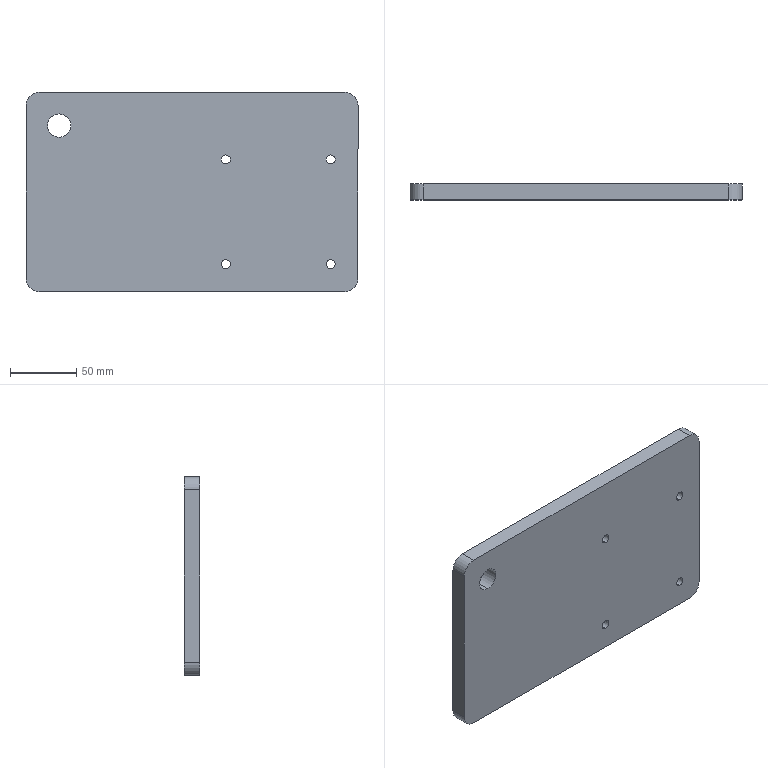Part | SolidWorks | features HoleWzd 4, ICE 2, Extrusion 1, Fillet 1 | 1 solid | 20 faces | box 250 x 12 x 150 mm | volume 444340 mm3 | cylinder 14 | plane 6 | commonest cylinder face diameters 6.8 x8 20 x4 17.5 x2
STEP:
#1=CARTESIAN_POINT('',(25.5,0.,-57.9));
#2=VERTEX_POINT('',#1);
#3=CARTESIAN_POINT('',(25.5,0.,-51.1));
#4=VERTEX_POINT('',#3);
#5=CARTESIAN_POINT('',(25.5,0.,-54.5));
#6=DIRECTION('',(0.,1.,0.));
#7=DIRECTION('',(0.,0.,1.));
#8=AXIS2_PLACEMENT_3D('',#5,#6,#7);
#9=CIRCLE('',#8,3.4);
#10=EDGE_CURVE('',#2,#4,#9,.T.);
#11=ORIENTED_EDGE('',*,*,#10,.F.);
#12=CARTESIAN_POINT('',(25.5,12.,-57.9));
#13=VERTEX_POINT('',#12);
#14=CARTESIAN_POINT('',(25.5,12.,-57.9));
#15=DIRECTION('',(0.,1.,0.));
#16=VECTOR('',#15,1000.);
#17=LINE('',#14,#16);
#18=EDGE_CURVE('',#2,#13,#17,.T.);
#19=ORIENTED_EDGE('',*,*,#18,.T.);
#20=CARTESIAN_POINT('',(25.5,12.,-51.1));
#21=VERTEX_POINT('',#20);
#22=CARTESIAN_POINT('',(25.5,12.,-54.5));
#23=DIRECTION('',(0.,1.,0.));
#24=DIRECTION('',(0.,0.,1.));
#25=AXIS2_PLACEMENT_3D('',#22,#23,#24);
#26=CIRCLE('',#25,3.4);
#27=EDGE_CURVE('',#13,#21,#26,.T.);
#28=ORIENTED_EDGE('',*,*,#27,.T.);
#29=CARTESIAN_POINT('',(25.5,12.,-51.1));
#30=DIRECTION('',(0.,1.,0.));
#31=VECTOR('',#30,1000.);
#32=LINE('',#29,#31);
#33=EDGE_CURVE('',#4,#21,#32,.T.);
#34=ORIENTED_EDGE('',*,*,#33,.F.);
#35=EDGE_LOOP('',(#11,#19,#28,#34));
#36=FACE_OUTER_BOUND('',#35,.T.);
#37=CARTESIAN_POINT('',(25.5,12.,-54.5));
#38=DIRECTION('',(0.,1.,0.));
#39=DIRECTION('',(0.,0.,1.));
#40=AXIS2_PLACEMENT_3D('',#37,#38,#39);
#41=CYLINDRICAL_SURFACE('',#40,3.4);
#42=ADVANCED_FACE('',(#36),#41,.F.);
#43=CARTESIAN_POINT('',(104.5,0.,-57.9));
#44=VERTEX_POINT('',#43);
#45=CARTESIAN_POINT('',(104.5,0.,-51.1));
#46=VERTEX_POINT('',#45);
#47=CARTESIAN_POINT('',(104.5,0.,-54.5));
#48=DIRECTION('',(0.,1.,0.));
#49=DIRECTION('',(0.,0.,1.));
#50=AXIS2_PLACEMENT_3D('',#47,#48,#49);
#51=CIRCLE('',#50,3.4);
#52=EDGE_CURVE('',#44,#46,#51,.T.);
#53=ORIENTED_EDGE('',*,*,#52,.F.);
#54=CARTESIAN_POINT('',(104.5,12.,-57.9));
#55=VERTEX_POINT('',#54);
#56=CARTESIAN_POINT('',(104.5,12.,-57.9));
#57=DIRECTION('',(0.,1.,0.));
#58=VECTOR('',#57,1000.);
#59=LINE('',#56,#58);
#60=EDGE_CURVE('',#44,#55,#59,.T.);
#61=ORIENTED_EDGE('',*,*,#60,.T.);
#62=CARTESIAN_POINT('',(104.5,12.,-51.1));
#63=VERTEX_POINT('',#62);
#64=CARTESIAN_POINT('',(104.5,12.,-54.5));
#65=DIRECTION('',(0.,1.,0.));
#66=DIRECTION('',(0.,0.,1.));
#67=AXIS2_PLACEMENT_3D('',#64,#65,#66);
#68=CIRCLE('',#67,3.4);
#69=EDGE_CURVE('',#55,#63,#68,.T.);
#70=ORIENTED_EDGE('',*,*,#69,.T.);
#71=CARTESIAN_POINT('',(104.5,12.,-51.1));
#72=DIRECTION('',(0.,1.,0.));
#73=VECTOR('',#72,1000.);
#74=LINE('',#71,#73);
#75=EDGE_CURVE('',#46,#63,#74,.T.);
#76=ORIENTED_EDGE('',*,*,#75,.F.);
#77=EDGE_LOOP('',(#53,#61,#70,#76));
#78=FACE_OUTER_BOUND('',#77,.T.);
#79=CARTESIAN_POINT('',(104.5,12.,-54.5));
#80=DIRECTION('',(0.,1.,0.));
#81=DIRECTION('',(0.,0.,1.));
#82=AXIS2_PLACEMENT_3D('',#79,#80,#81);
#83=CYLINDRICAL_SURFACE('',#82,3.4);
#84=ADVANCED_FACE('',(#78),#83,.F.);
#85=CARTESIAN_POINT('',(25.5,0.,21.1));
#86=VERTEX_POINT('',#85);
#87=CARTESIAN_POINT('',(25.5,0.,27.9));
#88=VERTEX_POINT('',#87);
#89=CARTESIAN_POINT('',(25.5,0.,24.5));
#90=DIRECTION('',(0.,1.,0.));
#91=DIRECTION('',(0.,0.,1.));
#92=AXIS2_PLACEMENT_3D('',#89,#90,#91);
#93=CIRCLE('',#92,3.4);
#94=EDGE_CURVE('',#86,#88,#93,.T.);
#95=ORIENTED_EDGE('',*,*,#94,.F.);
#96=CARTESIAN_POINT('',(25.5,12.,21.1));
#97=VERTEX_POINT('',#96);
#98=CARTESIAN_POINT('',(25.5,12.,21.1));
#99=DIRECTION('',(0.,1.,0.));
#100=VECTOR('',#99,1000.);
#101=LINE('',#98,#100);
#102=EDGE_CURVE('',#86,#97,#101,.T.);
#103=ORIENTED_EDGE('',*,*,#102,.T.);
#104=CARTESIAN_POINT('',(25.5,12.,27.9));
#105=VERTEX_POINT('',#104);
#106=CARTESIAN_POINT('',(25.5,12.,24.5));
#107=DIRECTION('',(0.,1.,0.));
#108=DIRECTION('',(0.,0.,1.));
#109=AXIS2_PLACEMENT_3D('',#106,#107,#108);
#110=CIRCLE('',#109,3.4);
#111=EDGE_CURVE('',#97,#105,#110,.T.);
#112=ORIENTED_EDGE('',*,*,#111,.T.);
#113=CARTESIAN_POINT('',(25.5,12.,27.9));
#114=DIRECTION('',(0.,1.,0.));
#115=VECTOR('',#114,1000.);
#116=LINE('',#113,#115);
#117=EDGE_CURVE('',#88,#105,#116,.T.);
#118=ORIENTED_EDGE('',*,*,#117,.F.);
#119=EDGE_LOOP('',(#95,#103,#112,#118));
#120=FACE_OUTER_BOUND('',#119,.T.);
#121=CARTESIAN_POINT('',(25.5,12.,24.5));
#122=DIRECTION('',(0.,1.,0.));
#123=DIRECTION('',(0.,0.,1.));
#124=AXIS2_PLACEMENT_3D('',#121,#122,#123);
#125=CYLINDRICAL_SURFACE('',#124,3.4);
#126=ADVANCED_FACE('',(#120),#125,.F.);
#127=CARTESIAN_POINT('',(104.5,0.,21.1));
#128=VERTEX_POINT('',#127);
#129=CARTESIAN_POINT('',(104.5,0.,27.9));
#130=VERTEX_POINT('',#129);
#131=CARTESIAN_POINT('',(104.5,0.,24.5));
#132=DIRECTION('',(0.,1.,0.));
#133=DIRECTION('',(0.,0.,1.));
#134=AXIS2_PLACEMENT_3D('',#131,#132,#133);
#135=CIRCLE('',#134,3.4);
#136=EDGE_CURVE('',#128,#130,#135,.T.);
#137=ORIENTED_EDGE('',*,*,#136,.F.);
#138=CARTESIAN_POINT('',(104.5,12.,21.1));
#139=VERTEX_POINT('',#138);
#140=CARTESIAN_POINT('',(104.5,12.,21.1));
#141=DIRECTION('',(0.,1.,0.));
#142=VECTOR('',#141,1000.);
#143=LINE('',#140,#142);
#144=EDGE_CURVE('',#128,#139,#143,.T.);
#145=ORIENTED_EDGE('',*,*,#144,.T.);
#146=CARTESIAN_POINT('',(104.5,12.,27.9));
#147=VERTEX_POINT('',#146);
#148=CARTESIAN_POINT('',(104.5,12.,24.5));
#149=DIRECTION('',(0.,1.,0.));
#150=DIRECTION('',(0.,0.,1.));
#151=AXIS2_PLACEMENT_3D('',#148,#149,#150);
#152=CIRCLE('',#151,3.4);
#153=EDGE_CURVE('',#139,#147,#152,.T.);
#154=ORIENTED_EDGE('',*,*,#153,.T.);
#155=CARTESIAN_POINT('',(104.5,12.,27.9));
#156=DIRECTION('',(0.,1.,0.));
#157=VECTOR('',#156,1000.);
#158=LINE('',#155,#157);
#159=EDGE_CURVE('',#130,#147,#158,.T.);
#160=ORIENTED_EDGE('',*,*,#159,.F.);
#161=EDGE_LOOP('',(#137,#145,#154,#160));
#162=FACE_OUTER_BOUND('',#161,.T.);
#163=CARTESIAN_POINT('',(104.5,12.,24.5));
#164=DIRECTION('',(0.,1.,0.));
#165=DIRECTION('',(0.,0.,1.));
#166=AXIS2_PLACEMENT_3D('',#163,#164,#165);
#167=CYLINDRICAL_SURFACE('',#166,3.4);
#168=ADVANCED_FACE('',(#162),#167,.F.);
#169=CARTESIAN_POINT('',(-100.,12.,58.75));
#170=VERTEX_POINT('',#169);
#171=CARTESIAN_POINT('',(-100.,12.,41.25));
#172=VERTEX_POINT('',#171);
#173=CARTESIAN_POINT('',(-100.,12.,50.));
#174=DIRECTION('',(0.,-1.,0.));
#175=DIRECTION('',(0.,0.,-1.));
#176=AXIS2_PLACEMENT_3D('',#173,#174,#175);
#177=CIRCLE('',#176,8.75);
#178=EDGE_CURVE('',#170,#172,#177,.T.);
#179=ORIENTED_EDGE('',*,*,#178,.F.);
#180=CARTESIAN_POINT('',(-100.,0.,58.75));
#181=VERTEX_POINT('',#180);
#182=CARTESIAN_POINT('',(-100.,0.,58.75));
#183=DIRECTION('',(0.,-1.,0.));
#184=VECTOR('',#183,1000.);
#185=LINE('',#182,#184);
#186=EDGE_CURVE('',#170,#181,#185,.T.);
#187=ORIENTED_EDGE('',*,*,#186,.T.);
#188=CARTESIAN_POINT('',(-100.,0.,41.25));
#189=VERTEX_POINT('',#188);
#190=CARTESIAN_POINT('',(-100.,0.,50.));
#191=DIRECTION('',(0.,-1.,0.));
#192=DIRECTION('',(0.,0.,-1.));
#193=AXIS2_PLACEMENT_3D('',#190,#191,#192);
#194=CIRCLE('',#193,8.75);
#195=EDGE_CURVE('',#181,#189,#194,.T.);
#196=ORIENTED_EDGE('',*,*,#195,.T.);
#197=CARTESIAN_POINT('',(-100.,0.,41.25));
#198=DIRECTION('',(0.,-1.,0.));
#199=VECTOR('',#198,1000.);
#200=LINE('',#197,#199);
#201=EDGE_CURVE('',#172,#189,#200,.T.);
#202=ORIENTED_EDGE('',*,*,#201,.F.);
#203=EDGE_LOOP('',(#179,#187,#196,#202));
#204=FACE_OUTER_BOUND('',#203,.T.);
#205=CARTESIAN_POINT('',(-100.,0.,50.));
#206=DIRECTION('',(0.,-1.,0.));
#207=DIRECTION('',(0.,0.,-1.));
#208=AXIS2_PLACEMENT_3D('',#205,#206,#207);
#209=CYLINDRICAL_SURFACE('',#208,8.75);
#210=ADVANCED_FACE('',(#204),#209,.F.);
#211=CARTESIAN_POINT('',(125.,0.,65.));
#212=VERTEX_POINT('',#211);
#213=CARTESIAN_POINT('',(125.,0.,-65.));
#214=VERTEX_POINT('',#213);
#215=CARTESIAN_POINT('',(125.,0.,-75.));
#216=DIRECTION('',(0.,0.,-1.));
#217=VECTOR('',#216,1000.);
#218=LINE('',#215,#217);
#219=EDGE_CURVE('',#212,#214,#218,.T.);
#220=ORIENTED_EDGE('',*,*,#219,.T.);
#221=CARTESIAN_POINT('',(125.,12.,-65.));
#222=VERTEX_POINT('',#221);
#223=CARTESIAN_POINT('',(125.,12.,-65.));
#224=DIRECTION('',(0.,1.,0.));
#225=VECTOR('',#224,1000.);
#226=LINE('',#223,#225);
#227=EDGE_CURVE('',#214,#222,#226,.T.);
#228=ORIENTED_EDGE('',*,*,#227,.T.);
#229=CARTESIAN_POINT('',(125.,12.,65.));
#230=VERTEX_POINT('',#229);
#231=CARTESIAN_POINT('',(125.,12.,-75.));
#232=DIRECTION('',(0.,0.,-1.));
#233=VECTOR('',#232,1000.);
#234=LINE('',#231,#233);
#235=EDGE_CURVE('',#230,#222,#234,.T.);
#236=ORIENTED_EDGE('',*,*,#235,.F.);
#237=CARTESIAN_POINT('',(125.,12.,65.));
#238=DIRECTION('',(0.,-1.,0.));
#239=VECTOR('',#238,1000.);
#240=LINE('',#237,#239);
#241=EDGE_CURVE('',#230,#212,#240,.T.);
#242=ORIENTED_EDGE('',*,*,#241,.T.);
#243=EDGE_LOOP('',(#220,#228,#236,#242));
#244=FACE_OUTER_BOUND('',#243,.T.);
#245=CARTESIAN_POINT('',(125.,12.,-75.));
#246=DIRECTION('',(-1.,0.,0.));
#247=DIRECTION('',(0.,0.,1.));
#248=AXIS2_PLACEMENT_3D('',#245,#246,#247);
#249=PLANE('',#248);
#250=ADVANCED_FACE('',(#244),#249,.F.);
#251=CARTESIAN_POINT('',(115.,0.,-75.));
#252=VERTEX_POINT('',#251);
#253=CARTESIAN_POINT('',(-115.,0.,-75.));
#254=VERTEX_POINT('',#253);
#255=CARTESIAN_POINT('',(-125.,0.,-75.));
#256=DIRECTION('',(-1.,0.,0.));
#257=VECTOR('',#256,1000.);
#258=LINE('',#255,#257);
#259=EDGE_CURVE('',#252,#254,#258,.T.);
#260=ORIENTED_EDGE('',*,*,#259,.T.);
#261=CARTESIAN_POINT('',(-115.,12.,-75.));
#262=VERTEX_POINT('',#261);
#263=CARTESIAN_POINT('',(-115.,12.,-75.));
#264=DIRECTION('',(0.,1.,0.));
#265=VECTOR('',#264,1000.);
#266=LINE('',#263,#265);
#267=EDGE_CURVE('',#254,#262,#266,.T.);
#268=ORIENTED_EDGE('',*,*,#267,.T.);
#269=CARTESIAN_POINT('',(115.,12.,-75.));
#270=VERTEX_POINT('',#269);
#271=CARTESIAN_POINT('',(-125.,12.,-75.));
#272=DIRECTION('',(-1.,0.,0.));
#273=VECTOR('',#272,1000.);
#274=LINE('',#271,#273);
#275=EDGE_CURVE('',#270,#262,#274,.T.);
#276=ORIENTED_EDGE('',*,*,#275,.F.);
#277=CARTESIAN_POINT('',(115.,12.,-75.));
#278=DIRECTION('',(0.,-1.,0.));
#279=VECTOR('',#278,1000.);
#280=LINE('',#277,#279);
#281=EDGE_CURVE('',#270,#252,#280,.T.);
#282=ORIENTED_EDGE('',*,*,#281,.T.);
#283=EDGE_LOOP('',(#260,#268,#276,#282));
#284=FACE_OUTER_BOUND('',#283,.T.);
#285=CARTESIAN_POINT('',(-125.,12.,-75.));
#286=DIRECTION('',(0.,0.,1.));
#287=DIRECTION('',(1.,0.,0.));
#288=AXIS2_PLACEMENT_3D('',#285,#286,#287);
#289=PLANE('',#288);
#290=ADVANCED_FACE('',(#284),#289,.F.);
#291=CARTESIAN_POINT('',(-125.,12.,-65.));
#292=VERTEX_POINT('',#291);
#293=CARTESIAN_POINT('',(-125.,12.,65.));
#294=VERTEX_POINT('',#293);
#295=CARTESIAN_POINT('',(-125.,12.,-75.));
#296=DIRECTION('',(0.,0.,1.));
#297=VECTOR('',#296,1000.);
#298=LINE('',#295,#297);
#299=EDGE_CURVE('',#292,#294,#298,.T.);
#300=ORIENTED_EDGE('',*,*,#299,.F.);
#301=CARTESIAN_POINT('',(-125.,0.,-65.));
#302=VERTEX_POINT('',#301);
#303=CARTESIAN_POINT('',(-125.,12.,-65.));
#304=DIRECTION('',(0.,-1.,0.));
#305=VECTOR('',#304,1000.);
#306=LINE('',#303,#305);
#307=EDGE_CURVE('',#292,#302,#306,.T.);
#308=ORIENTED_EDGE('',*,*,#307,.T.);
#309=CARTESIAN_POINT('',(-125.,0.,65.));
#310=VERTEX_POINT('',#309);
#311=CARTESIAN_POINT('',(-125.,0.,-75.));
#312=DIRECTION('',(0.,0.,1.));
#313=VECTOR('',#312,1000.);
#314=LINE('',#311,#313);
#315=EDGE_CURVE('',#302,#310,#314,.T.);
#316=ORIENTED_EDGE('',*,*,#315,.T.);
#317=CARTESIAN_POINT('',(-125.,12.,65.));
#318=DIRECTION('',(0.,1.,0.));
#319=VECTOR('',#318,1000.);
#320=LINE('',#317,#319);
#321=EDGE_CURVE('',#310,#294,#320,.T.);
#322=ORIENTED_EDGE('',*,*,#321,.T.);
#323=EDGE_LOOP('',(#300,#308,#316,#322));
#324=FACE_OUTER_BOUND('',#323,.T.);
#325=CARTESIAN_POINT('',(-125.,12.,-75.));
#326=DIRECTION('',(1.,0.,0.));
#327=DIRECTION('',(0.,0.,-1.));
#328=AXIS2_PLACEMENT_3D('',#325,#326,#327);
#329=PLANE('',#328);
#330=ADVANCED_FACE('',(#324),#329,.F.);
#331=CARTESIAN_POINT('',(-115.,0.,75.));
#332=VERTEX_POINT('',#331);
#333=CARTESIAN_POINT('',(115.,0.,75.));
#334=VERTEX_POINT('',#333);
#335=CARTESIAN_POINT('',(-125.,0.,75.));
#336=DIRECTION('',(1.,0.,0.));
#337=VECTOR('',#336,1000.);
#338=LINE('',#335,#337);
#339=EDGE_CURVE('',#332,#334,#338,.T.);
#340=ORIENTED_EDGE('',*,*,#339,.T.);
#341=CARTESIAN_POINT('',(115.,12.,75.));
#342=VERTEX_POINT('',#341);
#343=CARTESIAN_POINT('',(115.,12.,75.));
#344=DIRECTION('',(0.,1.,0.));
#345=VECTOR('',#344,1000.);
#346=LINE('',#343,#345);
#347=EDGE_CURVE('',#334,#342,#346,.T.);
#348=ORIENTED_EDGE('',*,*,#347,.T.);
#349=CARTESIAN_POINT('',(-115.,12.,75.));
#350=VERTEX_POINT('',#349);
#351=CARTESIAN_POINT('',(-125.,12.,75.));
#352=DIRECTION('',(1.,0.,0.));
#353=VECTOR('',#352,1000.);
#354=LINE('',#351,#353);
#355=EDGE_CURVE('',#350,#342,#354,.T.);
#356=ORIENTED_EDGE('',*,*,#355,.F.);
#357=CARTESIAN_POINT('',(-115.,12.,75.));
#358=DIRECTION('',(0.,-1.,0.));
#359=VECTOR('',#358,1000.);
#360=LINE('',#357,#359);
#361=EDGE_CURVE('',#350,#332,#360,.T.);
#362=ORIENTED_EDGE('',*,*,#361,.T.);
#363=EDGE_LOOP('',(#340,#348,#356,#362));
#364=FACE_OUTER_BOUND('',#363,.T.);
#365=CARTESIAN_POINT('',(-125.,12.,75.));
#366=DIRECTION('',(0.,0.,-1.));
#367=DIRECTION('',(-1.,0.,0.));
#368=AXIS2_PLACEMENT_3D('',#365,#366,#367);
#369=PLANE('',#368);
#370=ADVANCED_FACE('',(#364),#369,.F.);
#371=CARTESIAN_POINT('',(25.5,12.,-54.5));
#372=DIRECTION('',(0.,1.,0.));
#373=DIRECTION('',(0.,0.,1.));
#374=AXIS2_PLACEMENT_3D('',#371,#372,#373);
#375=CIRCLE('',#374,3.4);
#376=EDGE_CURVE('',#21,#13,#375,.T.);
#377=ORIENTED_EDGE('',*,*,#376,.F.);
#378=ORIENTED_EDGE('',*,*,#27,.F.);
#379=EDGE_LOOP('',(#377,#378));
#380=FACE_BOUND('',#379,.T.);
#381=CARTESIAN_POINT('',(104.5,12.,-54.5));
#382=DIRECTION('',(0.,1.,0.));
#383=DIRECTION('',(0.,0.,1.));
#384=AXIS2_PLACEMENT_3D('',#381,#382,#383);
#385=CIRCLE('',#384,3.4);
#386=EDGE_CURVE('',#63,#55,#385,.T.);
#387=ORIENTED_EDGE('',*,*,#386,.F.);
#388=ORIENTED_EDGE('',*,*,#69,.F.);
#389=EDGE_LOOP('',(#387,#388));
#390=FACE_BOUND('',#389,.T.);
#391=CARTESIAN_POINT('',(25.5,12.,24.5));
#392=DIRECTION('',(0.,1.,0.));
#393=DIRECTION('',(0.,0.,1.));
#394=AXIS2_PLACEMENT_3D('',#391,#392,#393);
#395=CIRCLE('',#394,3.4);
#396=EDGE_CURVE('',#105,#97,#395,.T.);
#397=ORIENTED_EDGE('',*,*,#396,.F.);
#398=ORIENTED_EDGE('',*,*,#111,.F.);
#399=EDGE_LOOP('',(#397,#398));
#400=FACE_BOUND('',#399,.T.);
#401=CARTESIAN_POINT('',(104.5,12.,24.5));
#402=DIRECTION('',(0.,1.,0.));
#403=DIRECTION('',(0.,0.,1.));
#404=AXIS2_PLACEMENT_3D('',#401,#402,#403);
#405=CIRCLE('',#404,3.4);
#406=EDGE_CURVE('',#147,#139,#405,.T.);
#407=ORIENTED_EDGE('',*,*,#406,.F.);
#408=ORIENTED_EDGE('',*,*,#153,.F.);
#409=EDGE_LOOP('',(#407,#408));
#410=FACE_BOUND('',#409,.T.);
#411=CARTESIAN_POINT('',(-100.,12.,50.));
#412=DIRECTION('',(0.,-1.,0.));
#413=DIRECTION('',(0.,0.,-1.));
#414=AXIS2_PLACEMENT_3D('',#411,#412,#413);
#415=CIRCLE('',#414,8.75);
#416=EDGE_CURVE('',#172,#170,#415,.T.);
#417=ORIENTED_EDGE('',*,*,#416,.T.);
#418=ORIENTED_EDGE('',*,*,#178,.T.);
#419=EDGE_LOOP('',(#417,#418));
#420=FACE_BOUND('',#419,.T.);
#421=ORIENTED_EDGE('',*,*,#275,.T.);
#422=CARTESIAN_POINT('',(-115.,12.,-65.));
#423=DIRECTION('',(0.,1.,0.));
#424=DIRECTION('',(0.,0.,1.));
#425=AXIS2_PLACEMENT_3D('',#422,#423,#424);
#426=CIRCLE('',#425,10.);
#427=EDGE_CURVE('',#262,#292,#426,.T.);
#428=ORIENTED_EDGE('',*,*,#427,.T.);
#429=ORIENTED_EDGE('',*,*,#299,.T.);
#430=CARTESIAN_POINT('',(-115.,12.,65.));
#431=DIRECTION('',(0.,1.,0.));
#432=DIRECTION('',(0.,0.,1.));
#433=AXIS2_PLACEMENT_3D('',#430,#431,#432);
#434=CIRCLE('',#433,10.);
#435=EDGE_CURVE('',#294,#350,#434,.T.);
#436=ORIENTED_EDGE('',*,*,#435,.T.);
#437=ORIENTED_EDGE('',*,*,#355,.T.);
#438=CARTESIAN_POINT('',(115.,12.,65.));
#439=DIRECTION('',(0.,1.,0.));
#440=DIRECTION('',(0.,0.,1.));
#441=AXIS2_PLACEMENT_3D('',#438,#439,#440);
#442=CIRCLE('',#441,10.);
#443=EDGE_CURVE('',#342,#230,#442,.T.);
#444=ORIENTED_EDGE('',*,*,#443,.T.);
#445=ORIENTED_EDGE('',*,*,#235,.T.);
#446=CARTESIAN_POINT('',(115.,12.,-65.));
#447=DIRECTION('',(0.,1.,0.));
#448=DIRECTION('',(0.,0.,1.));
#449=AXIS2_PLACEMENT_3D('',#446,#447,#448);
#450=CIRCLE('',#449,10.);
#451=EDGE_CURVE('',#222,#270,#450,.T.);
#452=ORIENTED_EDGE('',*,*,#451,.T.);
#453=EDGE_LOOP('',(#421,#428,#429,#436,#437,#444,#445,#452));
#454=FACE_OUTER_BOUND('',#453,.T.);
#455=CARTESIAN_POINT('',(0.,12.,0.));
#456=DIRECTION('',(0.,1.,0.));
#457=DIRECTION('',(0.,0.,1.));
#458=AXIS2_PLACEMENT_3D('',#455,#456,#457);
#459=PLANE('',#458);
#460=ADVANCED_FACE('',(#380,#390,#400,#410,#420,#454),#459,.T.);
#461=CARTESIAN_POINT('',(25.5,0.,-54.5));
#462=DIRECTION('',(0.,1.,0.));
#463=DIRECTION('',(0.,0.,1.));
#464=AXIS2_PLACEMENT_3D('',#461,#462,#463);
#465=CIRCLE('',#464,3.4);
#466=EDGE_CURVE('',#4,#2,#465,.T.);
#467=ORIENTED_EDGE('',*,*,#466,.T.);
#468=ORIENTED_EDGE('',*,*,#10,.T.);
#469=EDGE_LOOP('',(#467,#468));
#470=FACE_BOUND('',#469,.T.);
#471=CARTESIAN_POINT('',(104.5,0.,-54.5));
#472=DIRECTION('',(0.,1.,0.));
#473=DIRECTION('',(0.,0.,1.));
#474=AXIS2_PLACEMENT_3D('',#471,#472,#473);
#475=CIRCLE('',#474,3.4);
#476=EDGE_CURVE('',#46,#44,#475,.T.);
#477=ORIENTED_EDGE('',*,*,#476,.T.);
#478=ORIENTED_EDGE('',*,*,#52,.T.);
#479=EDGE_LOOP('',(#477,#478));
#480=FACE_BOUND('',#479,.T.);
#481=CARTESIAN_POINT('',(25.5,0.,24.5));
#482=DIRECTION('',(0.,1.,0.));
#483=DIRECTION('',(0.,0.,1.));
#484=AXIS2_PLACEMENT_3D('',#481,#482,#483);
#485=CIRCLE('',#484,3.4);
#486=EDGE_CURVE('',#88,#86,#485,.T.);
#487=ORIENTED_EDGE('',*,*,#486,.T.);
#488=ORIENTED_EDGE('',*,*,#94,.T.);
#489=EDGE_LOOP('',(#487,#488));
#490=FACE_BOUND('',#489,.T.);
#491=CARTESIAN_POINT('',(104.5,0.,24.5));
#492=DIRECTION('',(0.,1.,0.));
#493=DIRECTION('',(0.,0.,1.));
#494=AXIS2_PLACEMENT_3D('',#491,#492,#493);
#495=CIRCLE('',#494,3.4);
#496=EDGE_CURVE('',#130,#128,#495,.T.);
#497=ORIENTED_EDGE('',*,*,#496,.T.);
#498=ORIENTED_EDGE('',*,*,#136,.T.);
#499=EDGE_LOOP('',(#497,#498));
#500=FACE_BOUND('',#499,.T.);
#501=CARTESIAN_POINT('',(-100.,0.,50.));
#502=DIRECTION('',(0.,-1.,0.));
#503=DIRECTION('',(0.,0.,-1.));
#504=AXIS2_PLACEMENT_3D('',#501,#502,#503);
#505=CIRCLE('',#504,8.75);
#506=EDGE_CURVE('',#189,#181,#505,.T.);
#507=ORIENTED_EDGE('',*,*,#506,.F.);
#508=ORIENTED_EDGE('',*,*,#195,.F.);
#509=EDGE_LOOP('',(#507,#508));
#510=FACE_BOUND('',#509,.T.);
#511=ORIENTED_EDGE('',*,*,#315,.F.);
#512=CARTESIAN_POINT('',(-115.,0.,-65.));
#513=DIRECTION('',(0.,-1.,0.));
#514=DIRECTION('',(0.,0.,1.));
#515=AXIS2_PLACEMENT_3D('',#512,#513,#514);
#516=CIRCLE('',#515,10.);
#517=EDGE_CURVE('',#302,#254,#516,.T.);
#518=ORIENTED_EDGE('',*,*,#517,.T.);
#519=ORIENTED_EDGE('',*,*,#259,.F.);
#520=CARTESIAN_POINT('',(115.,0.,-65.));
#521=DIRECTION('',(0.,-1.,0.));
#522=DIRECTION('',(0.,0.,1.));
#523=AXIS2_PLACEMENT_3D('',#520,#521,#522);
#524=CIRCLE('',#523,10.);
#525=EDGE_CURVE('',#252,#214,#524,.T.);
#526=ORIENTED_EDGE('',*,*,#525,.T.);
#527=ORIENTED_EDGE('',*,*,#219,.F.);
#528=CARTESIAN_POINT('',(115.,0.,65.));
#529=DIRECTION('',(0.,-1.,0.));
#530=DIRECTION('',(0.,0.,1.));
#531=AXIS2_PLACEMENT_3D('',#528,#529,#530);
#532=CIRCLE('',#531,10.);
#533=EDGE_CURVE('',#212,#334,#532,.T.);
#534=ORIENTED_EDGE('',*,*,#533,.T.);
#535=ORIENTED_EDGE('',*,*,#339,.F.);
#536=CARTESIAN_POINT('',(-115.,0.,65.));
#537=DIRECTION('',(0.,-1.,0.));
#538=DIRECTION('',(0.,0.,1.));
#539=AXIS2_PLACEMENT_3D('',#536,#537,#538);
#540=CIRCLE('',#539,10.);
#541=EDGE_CURVE('',#332,#310,#540,.T.);
#542=ORIENTED_EDGE('',*,*,#541,.T.);
#543=EDGE_LOOP('',(#511,#518,#519,#526,#527,#534,#535,#542));
#544=FACE_OUTER_BOUND('',#543,.T.);
#545=CARTESIAN_POINT('',(0.,0.,0.));
#546=DIRECTION('',(0.,1.,0.));
#547=DIRECTION('',(0.,0.,1.));
#548=AXIS2_PLACEMENT_3D('',#545,#546,#547);
#549=PLANE('',#548);
#550=ADVANCED_FACE('',(#470,#480,#490,#500,#510,#544),#549,.F.);
#551=ORIENTED_EDGE('',*,*,#186,.F.);
#552=ORIENTED_EDGE('',*,*,#416,.F.);
#553=ORIENTED_EDGE('',*,*,#201,.T.);
#554=ORIENTED_EDGE('',*,*,#506,.T.);
#555=EDGE_LOOP('',(#551,#552,#553,#554));
#556=FACE_OUTER_BOUND('',#555,.T.);
#557=CARTESIAN_POINT('',(-100.,0.,50.));
#558=DIRECTION('',(0.,-1.,0.));
#559=DIRECTION('',(0.,0.,-1.));
#560=AXIS2_PLACEMENT_3D('',#557,#558,#559);
#561=CYLINDRICAL_SURFACE('',#560,8.75);
#562=ADVANCED_FACE('',(#556),#561,.F.);
#563=ORIENTED_EDGE('',*,*,#144,.F.);
#564=ORIENTED_EDGE('',*,*,#496,.F.);
#565=ORIENTED_EDGE('',*,*,#159,.T.);
#566=ORIENTED_EDGE('',*,*,#406,.T.);
#567=EDGE_LOOP('',(#563,#564,#565,#566));
#568=FACE_OUTER_BOUND('',#567,.T.);
#569=CARTESIAN_POINT('',(104.5,12.,24.5));
#570=DIRECTION('',(0.,1.,0.));
#571=DIRECTION('',(0.,0.,1.));
#572=AXIS2_PLACEMENT_3D('',#569,#570,#571);
#573=CYLINDRICAL_SURFACE('',#572,3.4);
#574=ADVANCED_FACE('',(#568),#573,.F.);
#575=ORIENTED_EDGE('',*,*,#102,.F.);
#576=ORIENTED_EDGE('',*,*,#486,.F.);
#577=ORIENTED_EDGE('',*,*,#117,.T.);
#578=ORIENTED_EDGE('',*,*,#396,.T.);
#579=EDGE_LOOP('',(#575,#576,#577,#578));
#580=FACE_OUTER_BOUND('',#579,.T.);
#581=CARTESIAN_POINT('',(25.5,12.,24.5));
#582=DIRECTION('',(0.,1.,0.));
#583=DIRECTION('',(0.,0.,1.));
#584=AXIS2_PLACEMENT_3D('',#581,#582,#583);
#585=CYLINDRICAL_SURFACE('',#584,3.4);
#586=ADVANCED_FACE('',(#580),#585,.F.);
#587=ORIENTED_EDGE('',*,*,#60,.F.);
#588=ORIENTED_EDGE('',*,*,#476,.F.);
#589=ORIENTED_EDGE('',*,*,#75,.T.);
#590=ORIENTED_EDGE('',*,*,#386,.T.);
#591=EDGE_LOOP('',(#587,#588,#589,#590));
#592=FACE_OUTER_BOUND('',#591,.T.);
#593=CARTESIAN_POINT('',(104.5,12.,-54.5));
#594=DIRECTION('',(0.,1.,0.));
#595=DIRECTION('',(0.,0.,1.));
#596=AXIS2_PLACEMENT_3D('',#593,#594,#595);
#597=CYLINDRICAL_SURFACE('',#596,3.4);
#598=ADVANCED_FACE('',(#592),#597,.F.);
#599=ORIENTED_EDGE('',*,*,#18,.F.);
#600=ORIENTED_EDGE('',*,*,#466,.F.);
#601=ORIENTED_EDGE('',*,*,#33,.T.);
#602=ORIENTED_EDGE('',*,*,#376,.T.);
#603=EDGE_LOOP('',(#599,#600,#601,#602));
#604=FACE_OUTER_BOUND('',#603,.T.);
#605=CARTESIAN_POINT('',(25.5,12.,-54.5));
#606=DIRECTION('',(0.,1.,0.));
#607=DIRECTION('',(0.,0.,1.));
#608=AXIS2_PLACEMENT_3D('',#605,#606,#607);
#609=CYLINDRICAL_SURFACE('',#608,3.4);
#610=ADVANCED_FACE('',(#604),#609,.F.);
#611=ORIENTED_EDGE('',*,*,#427,.F.);
#612=ORIENTED_EDGE('',*,*,#267,.F.);
#613=ORIENTED_EDGE('',*,*,#517,.F.);
#614=ORIENTED_EDGE('',*,*,#307,.F.);
#615=EDGE_LOOP('',(#611,#612,#613,#614));
#616=FACE_OUTER_BOUND('',#615,.T.);
#617=CARTESIAN_POINT('',(-115.,12.,-65.));
#618=DIRECTION('',(0.,-1.,0.));
#619=DIRECTION('',(0.,0.,-1.));
#620=AXIS2_PLACEMENT_3D('',#617,#618,#619);
#621=CYLINDRICAL_SURFACE('',#620,10.);
#622=ADVANCED_FACE('',(#616),#621,.T.);
#623=ORIENTED_EDGE('',*,*,#451,.F.);
#624=ORIENTED_EDGE('',*,*,#227,.F.);
#625=ORIENTED_EDGE('',*,*,#525,.F.);
#626=ORIENTED_EDGE('',*,*,#281,.F.);
#627=EDGE_LOOP('',(#623,#624,#625,#626));
#628=FACE_OUTER_BOUND('',#627,.T.);
#629=CARTESIAN_POINT('',(115.,12.,-65.));
#630=DIRECTION('',(0.,-1.,0.));
#631=DIRECTION('',(0.,0.,-1.));
#632=AXIS2_PLACEMENT_3D('',#629,#630,#631);
#633=CYLINDRICAL_SURFACE('',#632,10.);
#634=ADVANCED_FACE('',(#628),#633,.T.);
#635=ORIENTED_EDGE('',*,*,#443,.F.);
#636=ORIENTED_EDGE('',*,*,#347,.F.);
#637=ORIENTED_EDGE('',*,*,#533,.F.);
#638=ORIENTED_EDGE('',*,*,#241,.F.);
#639=EDGE_LOOP('',(#635,#636,#637,#638));
#640=FACE_OUTER_BOUND('',#639,.T.);
#641=CARTESIAN_POINT('',(115.,12.,65.));
#642=DIRECTION('',(0.,-1.,0.));
#643=DIRECTION('',(0.,0.,-1.));
#644=AXIS2_PLACEMENT_3D('',#641,#642,#643);
#645=CYLINDRICAL_SURFACE('',#644,10.);
#646=ADVANCED_FACE('',(#640),#645,.T.);
#647=ORIENTED_EDGE('',*,*,#435,.F.);
#648=ORIENTED_EDGE('',*,*,#321,.F.);
#649=ORIENTED_EDGE('',*,*,#541,.F.);
#650=ORIENTED_EDGE('',*,*,#361,.F.);
#651=EDGE_LOOP('',(#647,#648,#649,#650));
#652=FACE_OUTER_BOUND('',#651,.T.);
#653=CARTESIAN_POINT('',(-115.,12.,65.));
#654=DIRECTION('',(0.,-1.,0.));
#655=DIRECTION('',(0.,0.,-1.));
#656=AXIS2_PLACEMENT_3D('',#653,#654,#655);
#657=CYLINDRICAL_SURFACE('',#656,10.);
#658=ADVANCED_FACE('',(#652),#657,.T.);
#659=CLOSED_SHELL('',(#42,#84,#126,#168,#210,#250,#290,#330,#370,#460,#550,#562,#574,#586,#598,#610,#622,#634,#646,#658));
#660=MANIFOLD_SOLID_BREP('',#659);
#661=CARTESIAN_POINT('',(0.,0.,0.));
#662=DIRECTION('',(0.,0.,1.));
#663=DIRECTION('',(1.,0.,0.));
#664=AXIS2_PLACEMENT_3D('',#661,#662,#663);
#665=(LENGTH_UNIT()NAMED_UNIT(*)SI_UNIT(.MILLI.,.METRE.));
#666=UNCERTAINTY_MEASURE_WITH_UNIT(LENGTH_MEASURE(0.00001),#665,'','');
#667=(NAMED_UNIT(*)PLANE_ANGLE_UNIT()SI_UNIT($,.RADIAN.));
#668=(NAMED_UNIT(*)SI_UNIT($,.STERADIAN.)SOLID_ANGLE_UNIT());
#669=(GEOMETRIC_REPRESENTATION_CONTEXT(3)GLOBAL_UNCERTAINTY_ASSIGNED_CONTEXT((#666))GLOBAL_UNIT_ASSIGNED_CONTEXT((#665,#667,#668))REPRESENTATION_CONTEXT('',''));
#670=ADVANCED_BREP_SHAPE_REPRESENTATION('',(#660,#664),#669);